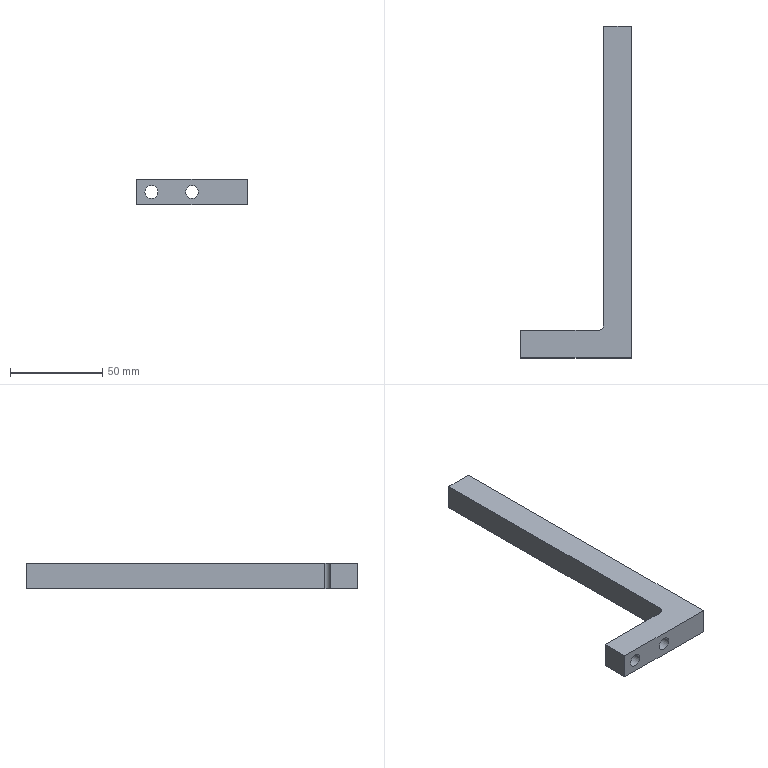Part | SolidWorks | features Extrusion 1, Fillet 1, ICE 1 | 1 solid | 13 faces | box 60 x 180 x 14 mm | volume 46123 mm3 | plane 8 | cylinder 5 | commonest cylinder face diameters 7 x4 6 x1
STEP:
#1=CARTESIAN_POINT('',(-55.5,0.,0.));
#2=VERTEX_POINT('',#1);
#3=CARTESIAN_POINT('',(-48.5,0.,0.));
#4=VERTEX_POINT('',#3);
#5=CARTESIAN_POINT('',(-52.,0.,0.));
#6=DIRECTION('',(0.,-1.,0.));
#7=DIRECTION('',(0.,0.,1.));
#8=AXIS2_PLACEMENT_3D('',#5,#6,#7);
#9=CIRCLE('',#8,3.5);
#10=EDGE_CURVE('',#2,#4,#9,.T.);
#11=ORIENTED_EDGE('',*,*,#10,.T.);
#12=CARTESIAN_POINT('',(-48.5,15.,0.));
#13=VERTEX_POINT('',#12);
#14=CARTESIAN_POINT('',(-48.5,-0.001,0.));
#15=DIRECTION('',(0.,1.,0.));
#16=VECTOR('',#15,1000.);
#17=LINE('',#14,#16);
#18=EDGE_CURVE('',#4,#13,#17,.T.);
#19=ORIENTED_EDGE('',*,*,#18,.T.);
#20=CARTESIAN_POINT('',(-55.5,15.,0.));
#21=VERTEX_POINT('',#20);
#22=CARTESIAN_POINT('',(-52.,15.,0.));
#23=DIRECTION('',(0.,1.,0.));
#24=DIRECTION('',(-1.,0.,0.));
#25=AXIS2_PLACEMENT_3D('',#22,#23,#24);
#26=CIRCLE('',#25,3.5);
#27=EDGE_CURVE('',#13,#21,#26,.T.);
#28=ORIENTED_EDGE('',*,*,#27,.T.);
#29=CARTESIAN_POINT('',(-55.5,-0.001,0.));
#30=DIRECTION('',(0.,1.,0.));
#31=VECTOR('',#30,1000.);
#32=LINE('',#29,#31);
#33=EDGE_CURVE('',#2,#21,#32,.T.);
#34=ORIENTED_EDGE('',*,*,#33,.F.);
#35=EDGE_LOOP('',(#11,#19,#28,#34));
#36=FACE_OUTER_BOUND('',#35,.T.);
#37=CARTESIAN_POINT('',(-52.,-0.001,0.));
#38=DIRECTION('',(0.,1.,0.));
#39=DIRECTION('',(-1.,0.,0.));
#40=AXIS2_PLACEMENT_3D('',#37,#38,#39);
#41=CYLINDRICAL_SURFACE('',#40,3.5);
#42=ADVANCED_FACE('',(#36),#41,.F.);
#43=CARTESIAN_POINT('',(-33.5,0.,0.));
#44=VERTEX_POINT('',#43);
#45=CARTESIAN_POINT('',(-26.5,0.,0.));
#46=VERTEX_POINT('',#45);
#47=CARTESIAN_POINT('',(-30.,0.,0.));
#48=DIRECTION('',(0.,-1.,0.));
#49=DIRECTION('',(0.,0.,1.));
#50=AXIS2_PLACEMENT_3D('',#47,#48,#49);
#51=CIRCLE('',#50,3.5);
#52=EDGE_CURVE('',#44,#46,#51,.T.);
#53=ORIENTED_EDGE('',*,*,#52,.T.);
#54=CARTESIAN_POINT('',(-26.5,15.,0.));
#55=VERTEX_POINT('',#54);
#56=CARTESIAN_POINT('',(-26.5,-0.001,0.));
#57=DIRECTION('',(0.,1.,0.));
#58=VECTOR('',#57,1000.);
#59=LINE('',#56,#58);
#60=EDGE_CURVE('',#46,#55,#59,.T.);
#61=ORIENTED_EDGE('',*,*,#60,.T.);
#62=CARTESIAN_POINT('',(-33.5,15.,0.));
#63=VERTEX_POINT('',#62);
#64=CARTESIAN_POINT('',(-30.,15.,0.));
#65=DIRECTION('',(0.,1.,0.));
#66=DIRECTION('',(-1.,0.,0.));
#67=AXIS2_PLACEMENT_3D('',#64,#65,#66);
#68=CIRCLE('',#67,3.5);
#69=EDGE_CURVE('',#55,#63,#68,.T.);
#70=ORIENTED_EDGE('',*,*,#69,.T.);
#71=CARTESIAN_POINT('',(-33.5,-0.001,0.));
#72=DIRECTION('',(0.,1.,0.));
#73=VECTOR('',#72,1000.);
#74=LINE('',#71,#73);
#75=EDGE_CURVE('',#44,#63,#74,.T.);
#76=ORIENTED_EDGE('',*,*,#75,.F.);
#77=EDGE_LOOP('',(#53,#61,#70,#76));
#78=FACE_OUTER_BOUND('',#77,.T.);
#79=CARTESIAN_POINT('',(-30.,-0.001,0.));
#80=DIRECTION('',(0.,1.,0.));
#81=DIRECTION('',(-1.,0.,0.));
#82=AXIS2_PLACEMENT_3D('',#79,#80,#81);
#83=CYLINDRICAL_SURFACE('',#82,3.5);
#84=ADVANCED_FACE('',(#78),#83,.F.);
#85=CARTESIAN_POINT('',(0.,0.,-7.));
#86=VERTEX_POINT('',#85);
#87=CARTESIAN_POINT('',(0.,180.,-7.));
#88=VERTEX_POINT('',#87);
#89=CARTESIAN_POINT('',(0.,180.,-7.));
#90=DIRECTION('',(0.,1.,0.));
#91=VECTOR('',#90,1000.);
#92=LINE('',#89,#91);
#93=EDGE_CURVE('',#86,#88,#92,.T.);
#94=ORIENTED_EDGE('',*,*,#93,.T.);
#95=CARTESIAN_POINT('',(0.,180.,7.));
#96=VERTEX_POINT('',#95);
#97=CARTESIAN_POINT('',(0.,180.,7.));
#98=DIRECTION('',(0.,0.,-1.));
#99=VECTOR('',#98,1000.);
#100=LINE('',#97,#99);
#101=EDGE_CURVE('',#96,#88,#100,.T.);
#102=ORIENTED_EDGE('',*,*,#101,.F.);
#103=CARTESIAN_POINT('',(0.,0.,7.));
#104=VERTEX_POINT('',#103);
#105=CARTESIAN_POINT('',(0.,180.,7.));
#106=DIRECTION('',(0.,1.,0.));
#107=VECTOR('',#106,1000.);
#108=LINE('',#105,#107);
#109=EDGE_CURVE('',#104,#96,#108,.T.);
#110=ORIENTED_EDGE('',*,*,#109,.F.);
#111=CARTESIAN_POINT('',(0.,0.,7.));
#112=DIRECTION('',(0.,0.,-1.));
#113=VECTOR('',#112,1000.);
#114=LINE('',#111,#113);
#115=EDGE_CURVE('',#104,#86,#114,.T.);
#116=ORIENTED_EDGE('',*,*,#115,.T.);
#117=EDGE_LOOP('',(#94,#102,#110,#116));
#118=FACE_OUTER_BOUND('',#117,.T.);
#119=CARTESIAN_POINT('',(0.,180.,7.));
#120=DIRECTION('',(-1.,0.,0.));
#121=DIRECTION('',(0.,-1.,0.));
#122=AXIS2_PLACEMENT_3D('',#119,#120,#121);
#123=PLANE('',#122);
#124=ADVANCED_FACE('',(#118),#123,.F.);
#125=CARTESIAN_POINT('',(-15.,180.,-7.));
#126=VERTEX_POINT('',#125);
#127=CARTESIAN_POINT('',(0.,180.,-7.));
#128=DIRECTION('',(-1.,0.,0.));
#129=VECTOR('',#128,1000.);
#130=LINE('',#127,#129);
#131=EDGE_CURVE('',#88,#126,#130,.T.);
#132=ORIENTED_EDGE('',*,*,#131,.T.);
#133=CARTESIAN_POINT('',(-15.,180.,7.));
#134=VERTEX_POINT('',#133);
#135=CARTESIAN_POINT('',(-15.,180.,7.));
#136=DIRECTION('',(0.,0.,-1.));
#137=VECTOR('',#136,1000.);
#138=LINE('',#135,#137);
#139=EDGE_CURVE('',#134,#126,#138,.T.);
#140=ORIENTED_EDGE('',*,*,#139,.F.);
#141=CARTESIAN_POINT('',(0.,180.,7.));
#142=DIRECTION('',(-1.,0.,0.));
#143=VECTOR('',#142,1000.);
#144=LINE('',#141,#143);
#145=EDGE_CURVE('',#96,#134,#144,.T.);
#146=ORIENTED_EDGE('',*,*,#145,.F.);
#147=ORIENTED_EDGE('',*,*,#101,.T.);
#148=EDGE_LOOP('',(#132,#140,#146,#147));
#149=FACE_OUTER_BOUND('',#148,.T.);
#150=CARTESIAN_POINT('',(0.,180.,7.));
#151=DIRECTION('',(0.,-1.,0.));
#152=DIRECTION('',(0.,0.,-1.));
#153=AXIS2_PLACEMENT_3D('',#150,#151,#152);
#154=PLANE('',#153);
#155=ADVANCED_FACE('',(#149),#154,.F.);
#156=CARTESIAN_POINT('',(-15.,18.,-7.));
#157=VERTEX_POINT('',#156);
#158=CARTESIAN_POINT('',(-15.,180.,-7.));
#159=DIRECTION('',(0.,-1.,0.));
#160=VECTOR('',#159,1000.);
#161=LINE('',#158,#160);
#162=EDGE_CURVE('',#126,#157,#161,.T.);
#163=ORIENTED_EDGE('',*,*,#162,.T.);
#164=CARTESIAN_POINT('',(-15.,18.,7.));
#165=VERTEX_POINT('',#164);
#166=CARTESIAN_POINT('',(-15.,18.,7.));
#167=DIRECTION('',(0.,0.,1.));
#168=VECTOR('',#167,1000.);
#169=LINE('',#166,#168);
#170=EDGE_CURVE('',#157,#165,#169,.T.);
#171=ORIENTED_EDGE('',*,*,#170,.T.);
#172=CARTESIAN_POINT('',(-15.,180.,7.));
#173=DIRECTION('',(0.,-1.,0.));
#174=VECTOR('',#173,1000.);
#175=LINE('',#172,#174);
#176=EDGE_CURVE('',#134,#165,#175,.T.);
#177=ORIENTED_EDGE('',*,*,#176,.F.);
#178=ORIENTED_EDGE('',*,*,#139,.T.);
#179=EDGE_LOOP('',(#163,#171,#177,#178));
#180=FACE_OUTER_BOUND('',#179,.T.);
#181=CARTESIAN_POINT('',(-15.,180.,7.));
#182=DIRECTION('',(1.,0.,0.));
#183=DIRECTION('',(0.,1.,0.));
#184=AXIS2_PLACEMENT_3D('',#181,#182,#183);
#185=PLANE('',#184);
#186=ADVANCED_FACE('',(#180),#185,.F.);
#187=CARTESIAN_POINT('',(-52.,15.,0.));
#188=DIRECTION('',(0.,1.,0.));
#189=DIRECTION('',(-1.,0.,0.));
#190=AXIS2_PLACEMENT_3D('',#187,#188,#189);
#191=CIRCLE('',#190,3.5);
#192=EDGE_CURVE('',#21,#13,#191,.T.);
#193=ORIENTED_EDGE('',*,*,#192,.F.);
#194=ORIENTED_EDGE('',*,*,#27,.F.);
#195=EDGE_LOOP('',(#193,#194));
#196=FACE_BOUND('',#195,.T.);
#197=CARTESIAN_POINT('',(-30.,15.,0.));
#198=DIRECTION('',(0.,1.,0.));
#199=DIRECTION('',(-1.,0.,0.));
#200=AXIS2_PLACEMENT_3D('',#197,#198,#199);
#201=CIRCLE('',#200,3.5);
#202=EDGE_CURVE('',#63,#55,#201,.T.);
#203=ORIENTED_EDGE('',*,*,#202,.F.);
#204=ORIENTED_EDGE('',*,*,#69,.F.);
#205=EDGE_LOOP('',(#203,#204));
#206=FACE_BOUND('',#205,.T.);
#207=CARTESIAN_POINT('',(-18.,15.,7.));
#208=VERTEX_POINT('',#207);
#209=CARTESIAN_POINT('',(-60.,15.,7.));
#210=VERTEX_POINT('',#209);
#211=CARTESIAN_POINT('',(-15.,15.,7.));
#212=DIRECTION('',(-1.,0.,0.));
#213=VECTOR('',#212,1000.);
#214=LINE('',#211,#213);
#215=EDGE_CURVE('',#208,#210,#214,.T.);
#216=ORIENTED_EDGE('',*,*,#215,.F.);
#217=CARTESIAN_POINT('',(-18.,15.,-7.));
#218=VERTEX_POINT('',#217);
#219=CARTESIAN_POINT('',(-18.,15.,-7.));
#220=DIRECTION('',(0.,0.,-1.));
#221=VECTOR('',#220,1000.);
#222=LINE('',#219,#221);
#223=EDGE_CURVE('',#208,#218,#222,.T.);
#224=ORIENTED_EDGE('',*,*,#223,.T.);
#225=CARTESIAN_POINT('',(-60.,15.,-7.));
#226=VERTEX_POINT('',#225);
#227=CARTESIAN_POINT('',(-15.,15.,-7.));
#228=DIRECTION('',(-1.,0.,0.));
#229=VECTOR('',#228,1000.);
#230=LINE('',#227,#229);
#231=EDGE_CURVE('',#218,#226,#230,.T.);
#232=ORIENTED_EDGE('',*,*,#231,.T.);
#233=CARTESIAN_POINT('',(-60.,15.,7.));
#234=DIRECTION('',(0.,0.,-1.));
#235=VECTOR('',#234,1000.);
#236=LINE('',#233,#235);
#237=EDGE_CURVE('',#210,#226,#236,.T.);
#238=ORIENTED_EDGE('',*,*,#237,.F.);
#239=EDGE_LOOP('',(#216,#224,#232,#238));
#240=FACE_OUTER_BOUND('',#239,.T.);
#241=CARTESIAN_POINT('',(-15.,15.,7.));
#242=DIRECTION('',(0.,-1.,0.));
#243=DIRECTION('',(1.,0.,0.));
#244=AXIS2_PLACEMENT_3D('',#241,#242,#243);
#245=PLANE('',#244);
#246=ADVANCED_FACE('',(#196,#206,#240),#245,.F.);
#247=CARTESIAN_POINT('',(-60.,0.,-7.));
#248=VERTEX_POINT('',#247);
#249=CARTESIAN_POINT('',(-60.,15.,-7.));
#250=DIRECTION('',(0.,-1.,0.));
#251=VECTOR('',#250,1000.);
#252=LINE('',#249,#251);
#253=EDGE_CURVE('',#226,#248,#252,.T.);
#254=ORIENTED_EDGE('',*,*,#253,.T.);
#255=CARTESIAN_POINT('',(-60.,0.,7.));
#256=VERTEX_POINT('',#255);
#257=CARTESIAN_POINT('',(-60.,0.,7.));
#258=DIRECTION('',(0.,0.,-1.));
#259=VECTOR('',#258,1000.);
#260=LINE('',#257,#259);
#261=EDGE_CURVE('',#256,#248,#260,.T.);
#262=ORIENTED_EDGE('',*,*,#261,.F.);
#263=CARTESIAN_POINT('',(-60.,15.,7.));
#264=DIRECTION('',(0.,-1.,0.));
#265=VECTOR('',#264,1000.);
#266=LINE('',#263,#265);
#267=EDGE_CURVE('',#210,#256,#266,.T.);
#268=ORIENTED_EDGE('',*,*,#267,.F.);
#269=ORIENTED_EDGE('',*,*,#237,.T.);
#270=EDGE_LOOP('',(#254,#262,#268,#269));
#271=FACE_OUTER_BOUND('',#270,.T.);
#272=CARTESIAN_POINT('',(-60.,15.,7.));
#273=DIRECTION('',(1.,0.,0.));
#274=DIRECTION('',(0.,1.,0.));
#275=AXIS2_PLACEMENT_3D('',#272,#273,#274);
#276=PLANE('',#275);
#277=ADVANCED_FACE('',(#271),#276,.F.);
#278=ORIENTED_EDGE('',*,*,#10,.F.);
#279=CARTESIAN_POINT('',(-52.,0.,0.));
#280=DIRECTION('',(0.,-1.,0.));
#281=DIRECTION('',(0.,0.,1.));
#282=AXIS2_PLACEMENT_3D('',#279,#280,#281);
#283=CIRCLE('',#282,3.5);
#284=EDGE_CURVE('',#4,#2,#283,.T.);
#285=ORIENTED_EDGE('',*,*,#284,.F.);
#286=EDGE_LOOP('',(#278,#285));
#287=FACE_BOUND('',#286,.T.);
#288=ORIENTED_EDGE('',*,*,#52,.F.);
#289=CARTESIAN_POINT('',(-30.,0.,0.));
#290=DIRECTION('',(0.,-1.,0.));
#291=DIRECTION('',(0.,0.,1.));
#292=AXIS2_PLACEMENT_3D('',#289,#290,#291);
#293=CIRCLE('',#292,3.5);
#294=EDGE_CURVE('',#46,#44,#293,.T.);
#295=ORIENTED_EDGE('',*,*,#294,.F.);
#296=EDGE_LOOP('',(#288,#295));
#297=FACE_BOUND('',#296,.T.);
#298=CARTESIAN_POINT('',(0.,0.,-7.));
#299=DIRECTION('',(1.,0.,0.));
#300=VECTOR('',#299,1000.);
#301=LINE('',#298,#300);
#302=EDGE_CURVE('',#248,#86,#301,.T.);
#303=ORIENTED_EDGE('',*,*,#302,.T.);
#304=ORIENTED_EDGE('',*,*,#115,.F.);
#305=CARTESIAN_POINT('',(0.,0.,7.));
#306=DIRECTION('',(1.,0.,0.));
#307=VECTOR('',#306,1000.);
#308=LINE('',#305,#307);
#309=EDGE_CURVE('',#256,#104,#308,.T.);
#310=ORIENTED_EDGE('',*,*,#309,.F.);
#311=ORIENTED_EDGE('',*,*,#261,.T.);
#312=EDGE_LOOP('',(#303,#304,#310,#311));
#313=FACE_OUTER_BOUND('',#312,.T.);
#314=CARTESIAN_POINT('',(0.,0.,7.));
#315=DIRECTION('',(0.,1.,0.));
#316=DIRECTION('',(0.,0.,1.));
#317=AXIS2_PLACEMENT_3D('',#314,#315,#316);
#318=PLANE('',#317);
#319=ADVANCED_FACE('',(#287,#297,#313),#318,.F.);
#320=ORIENTED_EDGE('',*,*,#109,.T.);
#321=ORIENTED_EDGE('',*,*,#145,.T.);
#322=ORIENTED_EDGE('',*,*,#176,.T.);
#323=CARTESIAN_POINT('',(-18.,18.,7.));
#324=DIRECTION('',(0.,0.,-1.));
#325=DIRECTION('',(-1.,0.,0.));
#326=AXIS2_PLACEMENT_3D('',#323,#324,#325);
#327=CIRCLE('',#326,3.);
#328=EDGE_CURVE('',#165,#208,#327,.T.);
#329=ORIENTED_EDGE('',*,*,#328,.T.);
#330=ORIENTED_EDGE('',*,*,#215,.T.);
#331=ORIENTED_EDGE('',*,*,#267,.T.);
#332=ORIENTED_EDGE('',*,*,#309,.T.);
#333=EDGE_LOOP('',(#320,#321,#322,#329,#330,#331,#332));
#334=FACE_OUTER_BOUND('',#333,.T.);
#335=CARTESIAN_POINT('',(0.,0.,7.));
#336=DIRECTION('',(0.,0.,-1.));
#337=DIRECTION('',(-1.,0.,0.));
#338=AXIS2_PLACEMENT_3D('',#335,#336,#337);
#339=PLANE('',#338);
#340=ADVANCED_FACE('',(#334),#339,.F.);
#341=ORIENTED_EDGE('',*,*,#93,.F.);
#342=ORIENTED_EDGE('',*,*,#302,.F.);
#343=ORIENTED_EDGE('',*,*,#253,.F.);
#344=ORIENTED_EDGE('',*,*,#231,.F.);
#345=CARTESIAN_POINT('',(-18.,18.,-7.));
#346=DIRECTION('',(0.,0.,1.));
#347=DIRECTION('',(-1.,0.,0.));
#348=AXIS2_PLACEMENT_3D('',#345,#346,#347);
#349=CIRCLE('',#348,3.);
#350=EDGE_CURVE('',#218,#157,#349,.T.);
#351=ORIENTED_EDGE('',*,*,#350,.T.);
#352=ORIENTED_EDGE('',*,*,#162,.F.);
#353=ORIENTED_EDGE('',*,*,#131,.F.);
#354=EDGE_LOOP('',(#341,#342,#343,#344,#351,#352,#353));
#355=FACE_OUTER_BOUND('',#354,.T.);
#356=CARTESIAN_POINT('',(0.,0.,-7.));
#357=DIRECTION('',(0.,0.,-1.));
#358=DIRECTION('',(-1.,0.,0.));
#359=AXIS2_PLACEMENT_3D('',#356,#357,#358);
#360=PLANE('',#359);
#361=ADVANCED_FACE('',(#355),#360,.T.);
#362=ORIENTED_EDGE('',*,*,#328,.F.);
#363=ORIENTED_EDGE('',*,*,#170,.F.);
#364=ORIENTED_EDGE('',*,*,#350,.F.);
#365=ORIENTED_EDGE('',*,*,#223,.F.);
#366=EDGE_LOOP('',(#362,#363,#364,#365));
#367=FACE_OUTER_BOUND('',#366,.T.);
#368=CARTESIAN_POINT('',(-18.,18.,7.));
#369=DIRECTION('',(0.,0.,1.));
#370=DIRECTION('',(1.,0.,0.));
#371=AXIS2_PLACEMENT_3D('',#368,#369,#370);
#372=CYLINDRICAL_SURFACE('',#371,3.);
#373=ADVANCED_FACE('',(#367),#372,.F.);
#374=ORIENTED_EDGE('',*,*,#60,.F.);
#375=ORIENTED_EDGE('',*,*,#294,.T.);
#376=ORIENTED_EDGE('',*,*,#75,.T.);
#377=ORIENTED_EDGE('',*,*,#202,.T.);
#378=EDGE_LOOP('',(#374,#375,#376,#377));
#379=FACE_OUTER_BOUND('',#378,.T.);
#380=CARTESIAN_POINT('',(-30.,-0.001,0.));
#381=DIRECTION('',(0.,1.,0.));
#382=DIRECTION('',(-1.,0.,0.));
#383=AXIS2_PLACEMENT_3D('',#380,#381,#382);
#384=CYLINDRICAL_SURFACE('',#383,3.5);
#385=ADVANCED_FACE('',(#379),#384,.F.);
#386=ORIENTED_EDGE('',*,*,#18,.F.);
#387=ORIENTED_EDGE('',*,*,#284,.T.);
#388=ORIENTED_EDGE('',*,*,#33,.T.);
#389=ORIENTED_EDGE('',*,*,#192,.T.);
#390=EDGE_LOOP('',(#386,#387,#388,#389));
#391=FACE_OUTER_BOUND('',#390,.T.);
#392=CARTESIAN_POINT('',(-52.,-0.001,0.));
#393=DIRECTION('',(0.,1.,0.));
#394=DIRECTION('',(-1.,0.,0.));
#395=AXIS2_PLACEMENT_3D('',#392,#393,#394);
#396=CYLINDRICAL_SURFACE('',#395,3.5);
#397=ADVANCED_FACE('',(#391),#396,.F.);
#398=CLOSED_SHELL('',(#42,#84,#124,#155,#186,#246,#277,#319,#340,#361,#373,#385,#397));
#399=MANIFOLD_SOLID_BREP('',#398);
#400=CARTESIAN_POINT('',(0.,0.,0.));
#401=DIRECTION('',(0.,0.,1.));
#402=DIRECTION('',(1.,0.,0.));
#403=AXIS2_PLACEMENT_3D('',#400,#401,#402);
#404=(LENGTH_UNIT()NAMED_UNIT(*)SI_UNIT(.MILLI.,.METRE.));
#405=UNCERTAINTY_MEASURE_WITH_UNIT(LENGTH_MEASURE(0.00001),#404,'','');
#406=(NAMED_UNIT(*)PLANE_ANGLE_UNIT()SI_UNIT($,.RADIAN.));
#407=(NAMED_UNIT(*)SI_UNIT($,.STERADIAN.)SOLID_ANGLE_UNIT());
#408=(GEOMETRIC_REPRESENTATION_CONTEXT(3)GLOBAL_UNCERTAINTY_ASSIGNED_CONTEXT((#405))GLOBAL_UNIT_ASSIGNED_CONTEXT((#404,#406,#407))REPRESENTATION_CONTEXT('',''));
#409=ADVANCED_BREP_SHAPE_REPRESENTATION('',(#399,#403),#408);